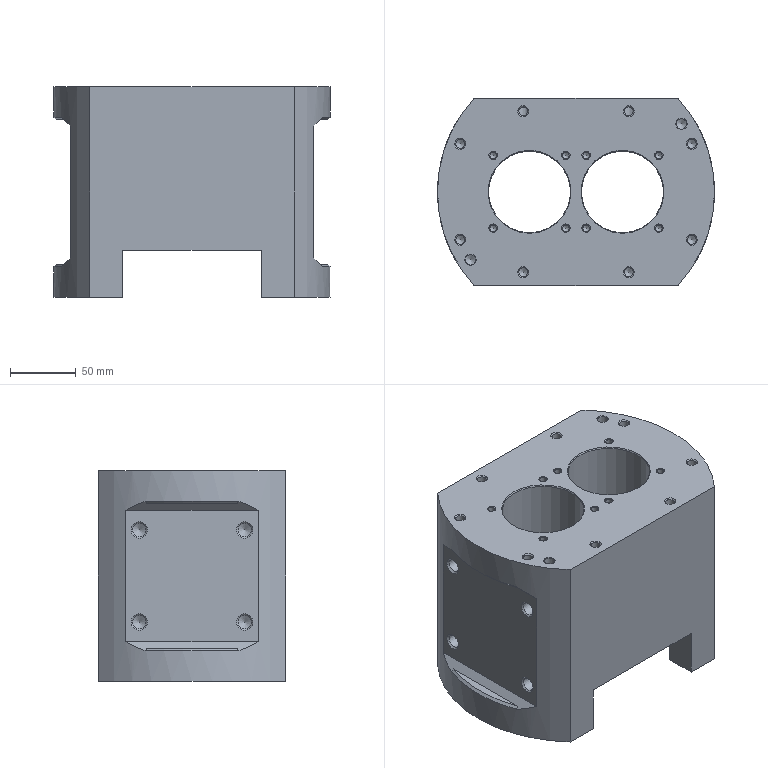NC program | NX | posted with a generic post | part box 210 x 142 x 160 mm
Whole program, first 1083 of 1408 lines:
N10 G17 G21 G94 G90
(FLOOR_WALL_COPY_COPY_COPY_COPY_1 , TOOL : D50)
N12 T02 M6
N14 G54
N16 G17 G0 G90 X-133. Y56.07 B0. C0. S2500 M3
N18 G43 Z30. H2
N20 Z4.
N22 G94 G1 Y70.997 Z0. F1000.
N24 X-108.901
N26 X108.901
N28 G2 X123.531 Y40.498 R130.
N30 G1 X-123.531
N32 G3 X-129.615 Y9.999 R130.
N34 G1 X129.615
N36 G2 X130. Y0.007 R130.
N38 G1 Y-0.007
N40 G2 X128.373 Y-20.501 R130.
N42 G1 X-128.373
N44 G3 X-119.578 Y-51. R130.
N46 G1 X119.578
N48 X122.578
N50 Z3.
N52 G0 Z30.
N54 M5
(DRILLING_COPY_2 , TOOL : ZXZ)
N56 T01 M6
N58 G54
N60 G17 G0 G90 X-87.769 Y36.355 B0. C0. S5000 M3
N62 G43 Z30. H1
N64 G94 G81 G98 Z-1. F250. R3.
N66 X-62.827 Y27.577
N68 X-40. Y61.
N70 X-7.673 Y27.577
N72 X7.673
N74 X40. Y61.
N76 X80. Y51.5
N78 X87.769 Y36.355
N80 X62.827 Y27.577
N82 X35.25 Y0.
N84 X62.827 Y-27.577
N86 X87.769 Y-36.355
N88 X40. Y-61.
N90 X7.673 Y-27.577
N92 X-7.673
N94 X-35.25 Y0.
N96 X-62.827 Y-27.577
N98 X-87.769 Y-36.355
N100 X-80. Y-51.5
N102 X-40. Y-61.
N104 G80
N106 G0 X-40. Y-61. Z30.
N108 M5
(DRILLING_COPY_2_COPY , TOOL : 6.8ZT)
N110 T16 M6
N112 G54
N114 G17 G0 G90 X-40. Y61. B0. C0. S2000 M3
N116 G43 Z30. H16
N118 G94 G83 G98 Z-24.742 F200. Q2. R3.
N120 X-87.769 Y36.355 Z-27.043
N122 Y-36.355
N124 X-40. Y-61.
N126 X40.
N128 X87.769 Y-36.355
N130 Y36.355
N132 X40. Y61. Z-24.742
N134 G80
N136 G0 X40. Y61. Z30.
N138 M5
(DRILLING_COPY_2_COPY_COPY_1 , TOOL : 5.2ZT)
N140 T15 M6
N142 G54
N144 G17 G0 G90 X62.827 Y27.577 B0. C0. S2000 M3
N146 G43 Z30. H15
N148 G94 G83 G98 Z-21.502 F200. Q2. R3.
N150 Y-27.577
N152 X7.673
N154 X-7.673
N156 X-62.827
N158 Y27.577
N160 X-7.673
N162 X7.673
N164 G80
N166 G0 X7.673 Y27.577 Z30.
N168 M5
(DRILLING_COPY_2_COPY_COPY_1_COPY_1 , TOOL : 7.8ZT)
N170 T17 M6
N172 G54
N174 G17 G0 G90 X80. Y51.5 B0. C0. S2000 M3
N176 G43 Z30. H17
N178 G94 G83 G98 Z-22.403 F200. Q2. R3.
N180 X-80. Y-51.5
N182 G80
N184 G0 X-80. Y-51.5 Z30.
N186 M5
(DRILLING_COPY_2_COPY_COPY_1_COPY_1_COPY , TOOL : 8.0JD)
N188 T18 M6
N190 G54
N192 G17 G0 G90 X80. Y51.5 B0. C0. S1000 M3
N194 G43 Z30. H18
N196 G94 G85 G98 Z-20. F40. R3.
N198 X-80. Y-51.5
N200 G80
N202 G0 X-80. Y-51.5 Z30.
N204 M5
(DRILLING_COPY_COPY_1_COPY , TOOL : 11.8ZT)
N206 T19 M6
N208 G54
N210 G17 G0 G90 X-35.25 Y0. B0. C0. S1025 M3
N212 G43 Z30. H19
N214 G94 G83 G98 Z-129.045 F150. Q2. R3.
N216 X35.25
N218 G80
N220 G0 X35.25 Y0. Z30.
N222 M5
(HOLE_MILLING , TOOL : D35R.5)
N224 T09 M6
N226 G54
N228 G17 G0 G90 X-35.25 Y0. B0. C0. S1500 M3
N230 G43 Z30. H9
N232 Z1.
N234 G94 G3 X-28.575 Y-6.675 R6.675 F1200.
N236 X-21.9 Y0. R6.675
N238 X-21.9 Y0. Z0.75 I-13.35 J0.
N240 X-21.9 Y0. Z0.5 I-13.35 J0.
N242 X-21.9 Y0. Z0.25 I-13.35 J0.
N244 X-21.9 Y0. Z0. I-13.35 J0.
N246 X-21.9 Y0. Z-0.25 I-13.35 J0.
N248 X-21.9 Y0. Z-0.5 I-13.35 J0.
N250 X-21.9 Y0. Z-0.75 I-13.35 J0.
N252 X-21.9 Y0. Z-1. I-13.35 J0.
N254 X-21.9 Y0. Z-1.25 I-13.35 J0.
N256 X-21.9 Y0. Z-1.5 I-13.35 J0.
N258 X-21.9 Y0. Z-1.75 I-13.35 J0.
N260 X-21.9 Y0. Z-2. I-13.35 J0.
N262 X-21.9 Y0. Z-2.25 I-13.35 J0.
N264 X-21.9 Y0. Z-2.5 I-13.35 J0.
N266 X-21.9 Y0. Z-2.75 I-13.35 J0.
N268 X-21.9 Y0. Z-3. I-13.35 J0.
N270 X-21.9 Y0. Z-3.25 I-13.35 J0.
N272 X-21.9 Y0. Z-3.5 I-13.35 J0.
N274 X-21.9 Y0. Z-3.75 I-13.35 J0.
N276 X-21.9 Y0. Z-4. I-13.35 J0.
N278 X-21.9 Y0. Z-4.25 I-13.35 J0.
N280 X-21.9 Y0. Z-4.5 I-13.35 J0.
N282 X-21.9 Y0. Z-4.75 I-13.35 J0.
N284 X-21.9 Y0. Z-5. I-13.35 J0.
N286 X-21.9 Y0. Z-5.25 I-13.35 J0.
N288 X-21.9 Y0. Z-5.5 I-13.35 J0.
N290 X-21.9 Y0. Z-5.75 I-13.35 J0.
N292 X-21.9 Y0. Z-6. I-13.35 J0.
N294 X-21.9 Y0. Z-6.25 I-13.35 J0.
N296 X-21.9 Y0. Z-6.5 I-13.35 J0.
N298 X-21.9 Y0. Z-6.75 I-13.35 J0.
N300 X-21.9 Y0. Z-7. I-13.35 J0.
N302 X-21.9 Y0. Z-7.25 I-13.35 J0.
N304 X-21.9 Y0. Z-7.5 I-13.35 J0.
N306 X-21.9 Y0. Z-7.75 I-13.35 J0.
N308 X-21.9 Y0. Z-8. I-13.35 J0.
N310 X-21.9 Y0. Z-8.25 I-13.35 J0.
N312 X-21.9 Y0. Z-8.5 I-13.35 J0.
N314 X-21.9 Y0. Z-8.75 I-13.35 J0.
N316 X-21.9 Y0. Z-9. I-13.35 J0.
N318 X-21.9 Y0. Z-9.25 I-13.35 J0.
N320 X-21.9 Y0. Z-9.5 I-13.35 J0.
N322 X-21.9 Y0. Z-9.75 I-13.35 J0.
N324 X-21.9 Y0. Z-10. I-13.35 J0.
N326 X-21.9 Y0. Z-10.25 I-13.35 J0.
N328 X-21.9 Y0. Z-10.5 I-13.35 J0.
N330 X-21.9 Y0. Z-10.75 I-13.35 J0.
N332 X-21.9 Y0. Z-11. I-13.35 J0.
N334 X-21.9 Y0. Z-11.25 I-13.35 J0.
N336 X-21.9 Y0. Z-11.5 I-13.35 J0.
N338 X-21.9 Y0. Z-11.75 I-13.35 J0.
N340 X-21.9 Y0. Z-12. I-13.35 J0.
N342 X-21.9 Y0. Z-12.25 I-13.35 J0.
N344 X-21.9 Y0. Z-12.5 I-13.35 J0.
N346 X-21.9 Y0. Z-12.75 I-13.35 J0.
N348 X-21.9 Y0. Z-13. I-13.35 J0.
N350 X-21.9 Y0. Z-13.25 I-13.35 J0.
N352 X-21.9 Y0. Z-13.5 I-13.35 J0.
N354 X-21.9 Y0. Z-13.75 I-13.35 J0.
N356 X-21.9 Y0. Z-14. I-13.35 J0.
N358 X-21.9 Y0. Z-14.25 I-13.35 J0.
N360 X-21.9 Y0. Z-14.5 I-13.35 J0.
N362 X-21.9 Y0. Z-14.75 I-13.35 J0.
N364 X-21.9 Y0. Z-15. I-13.35 J0.
N366 X-21.9 Y0. Z-15.25 I-13.35 J0.
N368 X-21.9 Y0. Z-15.5 I-13.35 J0.
N370 X-21.9 Y0. Z-15.75 I-13.35 J0.
N372 X-21.9 Y0. Z-16. I-13.35 J0.
N374 X-21.9 Y0. Z-16.25 I-13.35 J0.
N376 X-21.9 Y0. Z-16.5 I-13.35 J0.
N378 X-21.9 Y0. Z-16.75 I-13.35 J0.
N380 X-21.9 Y0. Z-17. I-13.35 J0.
N382 X-21.9 Y0. Z-17.25 I-13.35 J0.
N384 X-21.9 Y0. Z-17.5 I-13.35 J0.
N386 X-21.9 Y0. Z-17.75 I-13.35 J0.
N388 X-21.9 Y0. Z-18. I-13.35 J0.
N390 X-21.9 Y0. Z-18.25 I-13.35 J0.
N392 X-21.9 Y0. Z-18.5 I-13.35 J0.
N394 X-21.9 Y0. Z-18.75 I-13.35 J0.
N396 X-21.9 Y0. Z-19. I-13.35 J0.
N398 X-21.9 Y0. Z-19.25 I-13.35 J0.
N400 X-21.9 Y0. Z-19.5 I-13.35 J0.
N402 X-21.9 Y0. Z-19.75 I-13.35 J0.
N404 X-21.9 Y0. Z-20. I-13.35 J0.
N406 X-21.9 Y0. Z-20.25 I-13.35 J0.
N408 X-21.9 Y0. Z-20.5 I-13.35 J0.
N410 X-21.9 Y0. Z-20.75 I-13.35 J0.
N412 X-21.9 Y0. Z-21. I-13.35 J0.
N414 X-21.9 Y0. Z-21.25 I-13.35 J0.
N416 X-21.9 Y0. Z-21.5 I-13.35 J0.
N418 X-21.9 Y0. Z-21.75 I-13.35 J0.
N420 X-21.9 Y0. Z-22. I-13.35 J0.
N422 X-21.9 Y0. Z-22.25 I-13.35 J0.
N424 X-21.9 Y0. Z-22.5 I-13.35 J0.
N426 X-21.9 Y0. Z-22.75 I-13.35 J0.
N428 X-21.9 Y0. Z-23. I-13.35 J0.
N430 X-21.9 Y0. Z-23.25 I-13.35 J0.
N432 X-21.9 Y0. Z-23.5 I-13.35 J0.
N434 X-21.9 Y0. Z-23.75 I-13.35 J0.
N436 X-21.9 Y0. Z-24. I-13.35 J0.
N438 X-21.9 Y0. Z-24.25 I-13.35 J0.
N440 X-21.9 Y0. Z-24.5 I-13.35 J0.
N442 X-21.9 Y0. Z-24.75 I-13.35 J0.
N444 X-21.9 Y0. Z-25. I-13.35 J0.
N446 X-21.9 Y0. Z-25.25 I-13.35 J0.
N448 X-21.9 Y0. Z-25.5 I-13.35 J0.
N450 X-21.9 Y0. Z-25.75 I-13.35 J0.
N452 X-21.9 Y0. Z-26. I-13.35 J0.
N454 X-21.9 Y0. Z-26.25 I-13.35 J0.
N456 X-21.9 Y0. Z-26.5 I-13.35 J0.
N458 X-21.9 Y0. Z-26.75 I-13.35 J0.
N460 X-21.9 Y0. Z-27. I-13.35 J0.
N462 X-21.9 Y0. Z-27.25 I-13.35 J0.
N464 X-21.9 Y0. Z-27.5 I-13.35 J0.
N466 X-21.9 Y0. Z-27.75 I-13.35 J0.
N468 X-21.9 Y0. Z-28. I-13.35 J0.
N470 X-21.9 Y0. Z-28.25 I-13.35 J0.
N472 X-21.9 Y0. Z-28.5 I-13.35 J0.
N474 X-21.9 Y0. Z-28.75 I-13.35 J0.
N476 X-21.9 Y0. Z-29. I-13.35 J0.
N478 X-21.9 Y0. Z-29.25 I-13.35 J0.
N480 X-21.9 Y0. Z-29.5 I-13.35 J0.
N482 X-21.9 Y0. Z-29.75 I-13.35 J0.
N484 X-21.9 Y0. Z-30. I-13.35 J0.
N486 X-21.9 Y0. Z-30.25 I-13.35 J0.
N488 X-21.9 Y0. Z-30.5 I-13.35 J0.
N490 X-21.9 Y0. Z-30.75 I-13.35 J0.
N492 X-21.9 Y0. Z-31. I-13.35 J0.
N494 X-21.9 Y0. Z-31.25 I-13.35 J0.
N496 X-21.9 Y0. Z-31.5 I-13.35 J0.
N498 X-21.9 Y0. Z-31.75 I-13.35 J0.
N500 X-21.9 Y0. Z-32. I-13.35 J0.
N502 X-21.9 Y0. Z-32.25 I-13.35 J0.
N504 X-21.9 Y0. Z-32.5 I-13.35 J0.
N506 X-21.9 Y0. Z-32.75 I-13.35 J0.
N508 X-21.9 Y0. Z-33. I-13.35 J0.
N510 X-21.9 Y0. Z-33.25 I-13.35 J0.
N512 X-21.9 Y0. Z-33.5 I-13.35 J0.
N514 X-21.9 Y0. Z-33.75 I-13.35 J0.
N516 X-21.9 Y0. Z-34. I-13.35 J0.
N518 X-21.9 Y0. Z-34.25 I-13.35 J0.
N520 X-21.9 Y0. Z-34.5 I-13.35 J0.
N522 X-21.9 Y0. Z-34.75 I-13.35 J0.
N524 X-21.9 Y0. Z-35. I-13.35 J0.
N526 X-21.9 Y0. Z-35.25 I-13.35 J0.
N528 X-21.9 Y0. Z-35.5 I-13.35 J0.
N530 X-21.9 Y0. Z-35.75 I-13.35 J0.
N532 X-21.9 Y0. Z-36. I-13.35 J0.
N534 X-21.9 Y0. Z-36.25 I-13.35 J0.
N536 X-21.9 Y0. Z-36.5 I-13.35 J0.
N538 X-21.9 Y0. Z-36.75 I-13.35 J0.
N540 X-21.9 Y0. Z-37. I-13.35 J0.
N542 X-21.9 Y0. Z-37.25 I-13.35 J0.
N544 X-21.9 Y0. Z-37.5 I-13.35 J0.
N546 X-21.9 Y0. Z-37.75 I-13.35 J0.
N548 X-21.9 Y0. Z-38. I-13.35 J0.
N550 X-21.9 Y0. Z-38.25 I-13.35 J0.
N552 X-21.9 Y0. Z-38.5 I-13.35 J0.
N554 X-21.9 Y0. Z-38.75 I-13.35 J0.
N556 X-21.9 Y0. Z-39. I-13.35 J0.
N558 X-21.9 Y0. Z-39.25 I-13.35 J0.
N560 X-21.9 Y0. Z-39.5 I-13.35 J0.
N562 X-21.9 Y0. Z-39.75 I-13.35 J0.
N564 X-21.9 Y0. Z-40. I-13.35 J0.
N566 X-21.9 Y0. Z-40.25 I-13.35 J0.
N568 X-21.9 Y0. Z-40.5 I-13.35 J0.
N570 X-21.9 Y0. Z-40.75 I-13.35 J0.
N572 X-21.9 Y0. Z-41. I-13.35 J0.
N574 X-21.9 Y0. Z-41.25 I-13.35 J0.
N576 X-21.9 Y0. Z-41.5 I-13.35 J0.
N578 X-21.9 Y0. Z-41.75 I-13.35 J0.
N580 X-21.9 Y0. Z-42. I-13.35 J0.
N582 X-21.9 Y0. Z-42.25 I-13.35 J0.
N584 X-21.9 Y0. Z-42.5 I-13.35 J0.
N586 X-21.9 Y0. Z-42.75 I-13.35 J0.
N588 X-21.9 Y0. Z-43. I-13.35 J0.
N590 X-21.9 Y0. Z-43.25 I-13.35 J0.
N592 X-21.9 Y0. Z-43.5 I-13.35 J0.
N594 X-21.9 Y0. Z-43.75 I-13.35 J0.
N596 X-21.9 Y0. Z-44. I-13.35 J0.
N598 X-21.9 Y0. Z-44.25 I-13.35 J0.
N600 X-21.9 Y0. Z-44.5 I-13.35 J0.
N602 X-21.9 Y0. Z-44.75 I-13.35 J0.
N604 X-21.9 Y0. Z-45. I-13.35 J0.
N606 X-21.9 Y0. Z-45.25 I-13.35 J0.
N608 X-21.9 Y0. Z-45.5 I-13.35 J0.
N610 X-21.9 Y0. Z-45.75 I-13.35 J0.
N612 X-21.9 Y0. Z-46. I-13.35 J0.
N614 X-21.9 Y0. Z-46.25 I-13.35 J0.
N616 X-21.9 Y0. Z-46.5 I-13.35 J0.
N618 X-21.9 Y0. Z-46.75 I-13.35 J0.
N620 X-21.9 Y0. Z-47. I-13.35 J0.
N622 X-21.9 Y0. Z-47.25 I-13.35 J0.
N624 X-21.9 Y0. Z-47.5 I-13.35 J0.
N626 X-21.9 Y0. Z-47.75 I-13.35 J0.
N628 X-21.9 Y0. Z-48. I-13.35 J0.
N630 X-21.9 Y0. Z-48.25 I-13.35 J0.
N632 X-21.9 Y0. Z-48.5 I-13.35 J0.
N634 X-21.9 Y0. Z-48.75 I-13.35 J0.
N636 X-21.9 Y0. Z-49. I-13.35 J0.
N638 X-21.9 Y0. Z-49.25 I-13.35 J0.
N640 X-21.9 Y0. Z-49.5 I-13.35 J0.
N642 X-21.9 Y0. Z-49.75 I-13.35 J0.
N644 X-21.9 Y0. Z-50. I-13.35 J0.
N646 X-21.9 Y0. Z-50.25 I-13.35 J0.
N648 X-21.9 Y0. Z-50.5 I-13.35 J0.
N650 X-21.9 Y0. Z-50.75 I-13.35 J0.
N652 X-21.9 Y0. Z-51. I-13.35 J0.
N654 X-21.9 Y0. Z-51.25 I-13.35 J0.
N656 X-21.9 Y0. Z-51.5 I-13.35 J0.
N658 X-21.9 Y0. Z-51.75 I-13.35 J0.
N660 X-21.9 Y0. Z-52. I-13.35 J0.
N662 X-21.9 Y0. Z-52.25 I-13.35 J0.
N664 X-21.9 Y0. Z-52.5 I-13.35 J0.
N666 X-21.9 Y0. Z-52.75 I-13.35 J0.
N668 X-21.9 Y0. Z-53. I-13.35 J0.
N670 X-21.9 Y0. Z-53.25 I-13.35 J0.
N672 X-21.9 Y0. Z-53.5 I-13.35 J0.
N674 X-21.9 Y0. Z-53.75 I-13.35 J0.
N676 X-21.9 Y0. Z-54. I-13.35 J0.
N678 X-21.9 Y0. Z-54.25 I-13.35 J0.
N680 X-21.9 Y0. Z-54.5 I-13.35 J0.
N682 X-21.9 Y0. Z-54.75 I-13.35 J0.
N684 X-21.9 Y0. Z-55. I-13.35 J0.
N686 X-21.9 Y0. Z-55.25 I-13.35 J0.
N688 X-21.9 Y0. Z-55.5 I-13.35 J0.
N690 X-21.9 Y0. Z-55.75 I-13.35 J0.
N692 X-21.9 Y0. Z-56. I-13.35 J0.
N694 X-21.9 Y0. Z-56.25 I-13.35 J0.
N696 X-21.9 Y0. Z-56.5 I-13.35 J0.
N698 X-21.9 Y0. Z-56.75 I-13.35 J0.
N700 X-21.9 Y0. Z-57. I-13.35 J0.
N702 X-21.9 Y0. Z-57.25 I-13.35 J0.
N704 X-21.9 Y0. Z-57.5 I-13.35 J0.
N706 X-21.9 Y0. Z-57.75 I-13.35 J0.
N708 X-21.9 Y0. Z-58. I-13.35 J0.
N710 X-21.9 Y0. Z-58.25 I-13.35 J0.
N712 X-21.9 Y0. Z-58.5 I-13.35 J0.
N714 X-21.9 Y0. Z-58.75 I-13.35 J0.
N716 X-21.9 Y0. Z-59. I-13.35 J0.
N718 X-21.9 Y0. Z-59.25 I-13.35 J0.
N720 X-21.9 Y0. Z-59.5 I-13.35 J0.
N722 X-21.9 Y0. Z-59.75 I-13.35 J0.
N724 X-21.9 Y0. Z-60. I-13.35 J0.
N726 X-21.9 Y0. Z-60.25 I-13.35 J0.
N728 X-21.9 Y0. Z-60.5 I-13.35 J0.
N730 X-21.9 Y0. Z-60.75 I-13.35 J0.
N732 X-21.9 Y0. Z-61. I-13.35 J0.
N734 X-21.9 Y0. Z-61.25 I-13.35 J0.
N736 X-21.9 Y0. Z-61.5 I-13.35 J0.
N738 X-21.9 Y0. Z-61.75 I-13.35 J0.
N740 X-21.9 Y0. Z-62. I-13.35 J0.
N742 X-21.9 Y0. Z-62.25 I-13.35 J0.
N744 X-21.9 Y0. Z-62.5 I-13.35 J0.
N746 X-21.9 Y0. Z-62.75 I-13.35 J0.
N748 X-21.9 Y0. Z-63. I-13.35 J0.
N750 X-21.9 Y0. Z-63.25 I-13.35 J0.
N752 X-21.9 Y0. Z-63.5 I-13.35 J0.
N754 X-21.9 Y0. Z-63.75 I-13.35 J0.
N756 X-21.9 Y0. Z-64. I-13.35 J0.
N758 X-21.9 Y0. Z-64.25 I-13.35 J0.
N760 X-21.9 Y0. Z-64.5 I-13.35 J0.
N762 X-21.9 Y0. Z-64.75 I-13.35 J0.
N764 X-21.9 Y0. Z-65. I-13.35 J0.
N766 X-21.9 Y0. Z-65.25 I-13.35 J0.
N768 X-21.9 Y0. Z-65.5 I-13.35 J0.
N770 X-21.9 Y0. Z-65.75 I-13.35 J0.
N772 X-21.9 Y0. Z-66. I-13.35 J0.
N774 X-21.9 Y0. Z-66.25 I-13.35 J0.
N776 X-21.9 Y0. Z-66.5 I-13.35 J0.
N778 X-21.9 Y0. Z-66.75 I-13.35 J0.
N780 X-21.9 Y0. Z-67. I-13.35 J0.
N782 X-21.9 Y0. Z-67.25 I-13.35 J0.
N784 X-21.9 Y0. Z-67.5 I-13.35 J0.
N786 X-21.9 Y0. Z-67.75 I-13.35 J0.
N788 X-21.9 Y0. Z-68. I-13.35 J0.
N790 X-21.9 Y0. Z-68.25 I-13.35 J0.
N792 X-21.9 Y0. Z-68.5 I-13.35 J0.
N794 X-21.9 Y0. Z-68.75 I-13.35 J0.
N796 X-21.9 Y0. Z-69. I-13.35 J0.
N798 X-21.9 Y0. Z-69.25 I-13.35 J0.
N800 X-21.9 Y0. Z-69.5 I-13.35 J0.
N802 X-21.9 Y0. Z-69.75 I-13.35 J0.
N804 X-21.9 Y0. Z-70. I-13.35 J0.
N806 X-21.9 Y0. Z-70.25 I-13.35 J0.
N808 X-21.9 Y0. Z-70.5 I-13.35 J0.
N810 X-21.9 Y0. Z-70.75 I-13.35 J0.
N812 X-21.9 Y0. Z-71. I-13.35 J0.
N814 X-21.9 Y0. Z-71.25 I-13.35 J0.
N816 X-21.9 Y0. Z-71.5 I-13.35 J0.
N818 X-21.9 Y0. Z-71.75 I-13.35 J0.
N820 X-21.9 Y0. Z-72. I-13.35 J0.
N822 X-21.9 Y0. Z-72.25 I-13.35 J0.
N824 X-21.9 Y0. Z-72.5 I-13.35 J0.
N826 X-21.9 Y0. Z-72.75 I-13.35 J0.
N828 X-21.9 Y0. Z-73. I-13.35 J0.
N830 X-21.9 Y0. Z-73.25 I-13.35 J0.
N832 X-21.9 Y0. Z-73.5 I-13.35 J0.
N834 X-21.9 Y0. Z-73.75 I-13.35 J0.
N836 X-21.9 Y0. Z-74. I-13.35 J0.
N838 X-21.9 Y0. Z-74.25 I-13.35 J0.
N840 X-21.9 Y0. Z-74.5 I-13.35 J0.
N842 X-21.9 Y0. Z-74.75 I-13.35 J0.
N844 X-21.9 Y0. Z-75. I-13.35 J0.
N846 X-21.9 Y0. Z-75.25 I-13.35 J0.
N848 X-21.9 Y0. Z-75.5 I-13.35 J0.
N850 X-21.9 Y0. Z-75.75 I-13.35 J0.
N852 X-21.9 Y0. Z-76. I-13.35 J0.
N854 X-21.9 Y0. Z-76.25 I-13.35 J0.
N856 X-21.9 Y0. Z-76.5 I-13.35 J0.
N858 X-21.9 Y0. Z-76.75 I-13.35 J0.
N860 X-21.9 Y0. Z-77. I-13.35 J0.
N862 X-21.9 Y0. Z-77.25 I-13.35 J0.
N864 X-21.9 Y0. Z-77.5 I-13.35 J0.
N866 X-21.9 Y0. Z-77.75 I-13.35 J0.
N868 X-21.9 Y0. Z-78. I-13.35 J0.
N870 X-21.9 Y0. Z-78.25 I-13.35 J0.
N872 X-21.9 Y0. Z-78.5 I-13.35 J0.
N874 X-21.9 Y0. Z-78.75 I-13.35 J0.
N876 X-21.9 Y0. Z-79. I-13.35 J0.
N878 X-21.9 Y0. Z-79.25 I-13.35 J0.
N880 X-21.9 Y0. Z-79.5 I-13.35 J0.
N882 X-21.9 Y0. Z-79.75 I-13.35 J0.
N884 X-21.9 Y0. Z-80. I-13.35 J0.
N886 X-21.9 Y0. Z-80.25 I-13.35 J0.
N888 X-21.9 Y0. Z-80.5 I-13.35 J0.
N890 X-21.9 Y0. Z-80.75 I-13.35 J0.
N892 X-21.9 Y0. Z-81. I-13.35 J0.
N894 X-21.9 Y0. Z-81.25 I-13.35 J0.
N896 X-21.9 Y0. Z-81.5 I-13.35 J0.
N898 X-21.9 Y0. Z-81.75 I-13.35 J0.
N900 X-21.9 Y0. Z-82. I-13.35 J0.
N902 X-21.9 Y0. Z-82.25 I-13.35 J0.
N904 X-21.9 Y0. Z-82.5 I-13.35 J0.
N906 X-21.9 Y0. Z-82.75 I-13.35 J0.
N908 X-21.9 Y0. Z-83. I-13.35 J0.
N910 X-21.9 Y0. Z-83.25 I-13.35 J0.
N912 X-21.9 Y0. Z-83.5 I-13.35 J0.
N914 X-21.9 Y0. Z-83.75 I-13.35 J0.
N916 X-21.9 Y0. Z-84. I-13.35 J0.
N918 X-21.9 Y0. Z-84.25 I-13.35 J0.
N920 X-21.9 Y0. Z-84.5 I-13.35 J0.
N922 X-21.9 Y0. Z-84.75 I-13.35 J0.
N924 X-21.9 Y0. Z-85. I-13.35 J0.
N926 X-21.9 Y0. Z-85.25 I-13.35 J0.
N928 X-21.9 Y0. Z-85.5 I-13.35 J0.
N930 X-21.9 Y0. Z-85.75 I-13.35 J0.
N932 X-21.9 Y0. Z-86. I-13.35 J0.
N934 X-21.9 Y0. Z-86.25 I-13.35 J0.
N936 X-21.9 Y0. Z-86.5 I-13.35 J0.
N938 X-21.9 Y0. Z-86.75 I-13.35 J0.
N940 X-21.9 Y0. Z-87. I-13.35 J0.
N942 X-21.9 Y0. Z-87.25 I-13.35 J0.
N944 X-21.9 Y0. Z-87.5 I-13.35 J0.
N946 X-21.9 Y0. Z-87.75 I-13.35 J0.
N948 X-21.9 Y0. Z-88. I-13.35 J0.
N950 X-21.9 Y0. Z-88.25 I-13.35 J0.
N952 X-21.9 Y0. Z-88.5 I-13.35 J0.
N954 X-21.9 Y0. Z-88.75 I-13.35 J0.
N956 X-21.9 Y0. Z-89. I-13.35 J0.
N958 X-21.9 Y0. Z-89.25 I-13.35 J0.
N960 X-21.9 Y0. Z-89.5 I-13.35 J0.
N962 X-21.9 Y0. Z-89.75 I-13.35 J0.
N964 X-21.9 Y0. Z-90. I-13.35 J0.
N966 X-21.9 Y0. Z-90.25 I-13.35 J0.
N968 X-21.9 Y0. Z-90.5 I-13.35 J0.
N970 X-21.9 Y0. Z-90.75 I-13.35 J0.
N972 X-21.9 Y0. Z-91. I-13.35 J0.
N974 X-21.9 Y0. Z-91.25 I-13.35 J0.
N976 X-21.9 Y0. Z-91.5 I-13.35 J0.
N978 X-21.9 Y0. Z-91.75 I-13.35 J0.
N980 X-21.9 Y0. Z-92. I-13.35 J0.
N982 X-21.9 Y0. Z-92.25 I-13.35 J0.
N984 X-21.9 Y0. Z-92.5 I-13.35 J0.
N986 X-21.9 Y0. Z-92.75 I-13.35 J0.
N988 X-21.9 Y0. Z-93. I-13.35 J0.
N990 X-21.9 Y0. Z-93.25 I-13.35 J0.
N992 X-21.9 Y0. Z-93.5 I-13.35 J0.
N994 X-21.9 Y0. Z-93.75 I-13.35 J0.
N996 X-21.9 Y0. Z-94. I-13.35 J0.
N998 X-21.9 Y0. Z-94.25 I-13.35 J0.
N1000 X-21.9 Y0. Z-94.5 I-13.35 J0.
N1002 X-21.9 Y0. Z-94.75 I-13.35 J0.
N1004 X-21.9 Y0. Z-95. I-13.35 J0.
N1006 X-21.9 Y0. Z-95.25 I-13.35 J0.
N1008 X-21.9 Y0. Z-95.5 I-13.35 J0.
N1010 X-21.9 Y0. Z-95.75 I-13.35 J0.
N1012 X-21.9 Y0. Z-96. I-13.35 J0.
N1014 X-21.9 Y0. Z-96.25 I-13.35 J0.
N1016 X-21.9 Y0. Z-96.5 I-13.35 J0.
N1018 X-21.9 Y0. Z-96.75 I-13.35 J0.
N1020 X-21.9 Y0. Z-97. I-13.35 J0.
N1022 X-21.9 Y0. Z-97.25 I-13.35 J0.
N1024 X-21.9 Y0. Z-97.5 I-13.35 J0.
N1026 X-21.9 Y0. Z-97.75 I-13.35 J0.
N1028 X-21.9 Y0. Z-98. I-13.35 J0.
N1030 X-21.9 Y0. Z-98.25 I-13.35 J0.
N1032 X-21.9 Y0. Z-98.5 I-13.35 J0.
N1034 X-21.9 Y0. Z-98.75 I-13.35 J0.
N1036 X-21.9 Y0. Z-99. I-13.35 J0.
N1038 X-21.9 Y0. Z-99.25 I-13.35 J0.
N1040 X-21.9 Y0. Z-99.5 I-13.35 J0.
N1042 X-21.9 Y0. Z-99.75 I-13.35 J0.
N1044 X-21.9 Y0. Z-100. I-13.35 J0.
N1046 X-21.9 Y0. Z-100.25 I-13.35 J0.
N1048 X-21.9 Y0. Z-100.5 I-13.35 J0.
N1050 X-21.9 Y0. Z-100.75 I-13.35 J0.
N1052 X-21.9 Y0. Z-101. I-13.35 J0.
N1054 X-21.9 Y0. Z-101.25 I-13.35 J0.
N1056 X-21.9 Y0. Z-101.5 I-13.35 J0.
N1058 X-21.9 Y0. Z-101.75 I-13.35 J0.
N1060 X-21.9 Y0. Z-102. I-13.35 J0.
N1062 X-21.9 Y0. Z-102.25 I-13.35 J0.
N1064 X-21.9 Y0. Z-102.5 I-13.35 J0.
N1066 X-21.9 Y0. Z-102.75 I-13.35 J0.
N1068 X-21.9 Y0. Z-103. I-13.35 J0.
N1070 X-21.9 Y0. Z-103.25 I-13.35 J0.
N1072 X-21.9 Y0. Z-103.5 I-13.35 J0.
N1074 X-21.9 Y0. Z-103.75 I-13.35 J0.
N1076 X-21.9 Y0. Z-104. I-13.35 J0.
N1078 X-21.9 Y0. Z-104.25 I-13.35 J0.
N1080 X-21.9 Y0. Z-104.5 I-13.35 J0.
N1082 X-21.9 Y0. Z-104.75 I-13.35 J0.
N1084 X-21.9 Y0. Z-105. I-13.35 J0.
N1086 X-21.9 Y0. Z-105.25 I-13.35 J0.
N1088 X-21.9 Y0. Z-105.5 I-13.35 J0.
N1090 X-21.9 Y0. Z-105.75 I-13.35 J0.
N1092 X-21.9 Y0. Z-106. I-13.35 J0.
N1094 X-21.9 Y0. Z-106.25 I-13.35 J0.
N1096 X-21.9 Y0. Z-106.5 I-13.35 J0.
N1098 X-21.9 Y0. Z-106.75 I-13.35 J0.
N1100 X-21.9 Y0. Z-107. I-13.35 J0.
N1102 X-21.9 Y0. Z-107.25 I-13.35 J0.
N1104 X-21.9 Y0. Z-107.5 I-13.35 J0.
N1106 X-21.9 Y0. Z-107.75 I-13.35 J0.
N1108 X-21.9 Y0. Z-108. I-13.35 J0.
N1110 X-21.9 Y0. Z-108.25 I-13.35 J0.
N1112 X-21.9 Y0. Z-108.5 I-13.35 J0.
N1114 X-21.9 Y0. Z-108.75 I-13.35 J0.
N1116 X-21.9 Y0. Z-109. I-13.35 J0.
N1118 X-21.9 Y0. Z-109.25 I-13.35 J0.
N1120 X-21.9 Y0. Z-109.5 I-13.35 J0.
N1122 X-21.9 Y0. Z-109.75 I-13.35 J0.
N1124 X-21.9 Y0. Z-110. I-13.35 J0.
N1126 X-21.9 Y0. Z-110.25 I-13.35 J0.
N1128 X-21.9 Y0. Z-110.5 I-13.35 J0.
N1130 X-21.9 Y0. Z-110.75 I-13.35 J0.
N1132 X-21.9 Y0. Z-111. I-13.35 J0.
N1134 X-21.9 Y0. Z-111.25 I-13.35 J0.
N1136 X-21.9 Y0. Z-111.5 I-13.35 J0.
N1138 X-21.9 Y0. Z-111.75 I-13.35 J0.
N1140 X-21.9 Y0. Z-112. I-13.35 J0.
N1142 X-21.9 Y0. Z-112.25 I-13.35 J0.
N1144 X-21.9 Y0. Z-112.5 I-13.35 J0.
N1146 X-21.9 Y0. Z-112.75 I-13.35 J0.
N1148 X-21.9 Y0. Z-113. I-13.35 J0.
N1150 X-21.9 Y0. Z-113.25 I-13.35 J0.
N1152 X-21.9 Y0. Z-113.5 I-13.35 J0.
N1154 X-21.9 Y0. Z-113.75 I-13.35 J0.
N1156 X-21.9 Y0. Z-114. I-13.35 J0.
N1158 X-21.9 Y0. Z-114.25 I-13.35 J0.
N1160 X-21.9 Y0. Z-114.5 I-13.35 J0.
N1162 X-21.9 Y0. Z-114.75 I-13.35 J0.
N1164 X-21.9 Y0. Z-115. I-13.35 J0.
N1166 X-21.9 Y0. Z-115.25 I-13.35 J0.
N1168 X-21.9 Y0. Z-115.5 I-13.35 J0.
N1170 X-21.9 Y0. Z-115.75 I-13.35 J0.
N1172 X-21.9 Y0. Z-116. I-13.35 J0.
N1174 X-21.9 Y0. Z-116.25 I-13.35 J0.
N1176 X-21.9 Y0. Z-116.5 I-13.35 J0.
N1178 X-21.9 Y0. Z-116.75 I-13.35 J0.
N1180 X-21.9 Y0. Z-117. I-13.35 J0.
N1182 X-21.9 Y0. Z-117.25 I-13.35 J0.
N1184 X-21.9 Y0. Z-117.5 I-13.35 J0.
N1186 X-21.9 Y0. Z-117.75 I-13.35 J0.
N1188 X-21.9 Y0. Z-118. I-13.35 J0.
N1190 X-21.9 Y0. Z-118.25 I-13.35 J0.
N1192 X-21.9 Y0. Z-118.5 I-13.35 J0.
N1194 X-21.9 Y0. Z-118.75 I-13.35 J0.
N1196 X-21.9 Y0. Z-119. I-13.35 J0.
N1198 X-21.9 Y0. Z-119.25 I-13.35 J0.
N1200 X-21.9 Y0. Z-119.5 I-13.35 J0.
N1202 X-21.9 Y0. Z-119.75 I-13.35 J0.
N1204 X-21.9 Y0. Z-120. I-13.35 J0.
N1206 X-21.9 Y0. Z-120.25 I-13.35 J0.
N1208 X-21.9 Y0. Z-120.5 I-13.35 J0.
N1210 X-21.9 Y0. Z-120.75 I-13.35 J0.
N1212 X-21.9 Y0. Z-121. I-13.35 J0.
N1214 X-21.9 Y0. Z-121.25 I-13.35 J0.
N1216 X-21.9 Y0. Z-121.5 I-13.35 J0.
N1218 X-21.9 Y0. Z-121.75 I-13.35 J0.
N1220 X-21.9 Y0. Z-122. I-13.35 J0.
N1222 X-21.9 Y0. Z-122.25 I-13.35 J0.
N1224 X-21.9 Y0. Z-122.5 I-13.35 J0.
N1226 X-21.9 Y0. Z-122.75 I-13.35 J0.
N1228 X-21.9 Y0. Z-123. I-13.35 J0.
N1230 X-21.9 Y0. Z-123.25 I-13.35 J0.
N1232 X-21.9 Y0. Z-123.5 I-13.35 J0.
N1234 X-21.9 Y0. Z-123.75 I-13.35 J0.
N1236 X-21.9 Y0. Z-124. I-13.35 J0.
N1238 X-21.9 Y0. Z-124.25 I-13.35 J0.
N1240 X-21.9 Y0. Z-124.5 I-13.35 J0.
N1242 X-21.9 Y0. Z-124.75 I-13.35 J0.
N1244 X-21.9 Y0. Z-125. I-13.35 J0.
N1246 X-21.9 Y0. Z-125.25 I-13.35 J0.
N1248 X-21.9 Y0. Z-125.5 I-13.35 J0.
N1250 X-21.9 Y0. Z-125.75 I-13.35 J0.
N1252 X-21.9 Y0. Z-126. I-13.35 J0.
N1254 X-35.25 Y13.35 R13.35
N1256 X-21.9 Y0. R-13.35
N1258 X-28.575 Y6.675 R6.675
N1260 X-35.25 Y0. R6.675
N1262 G0 Z30.
N1264 X35.25
N1266 Z1.
N1268 G3 X41.925 Y-6.675 R6.675
N1270 X48.6 Y0. R6.675
N1272 X48.6 Y0. Z0.75 I-13.35 J0.
N1274 X48.6 Y0. Z0.5 I-13.35 J0.
N1276 X48.6 Y0. Z0.25 I-13.35 J0.
N1278 X48.6 Y0. Z0. I-13.35 J0.
N1280 X48.6 Y0. Z-0.25 I-13.35 J0.
N1282 X48.6 Y0. Z-0.5 I-13.35 J0.
N1284 X48.6 Y0. Z-0.75 I-13.35 J0.
N1286 X48.6 Y0. Z-1. I-13.35 J0.
N1288 X48.6 Y0. Z-1.25 I-13.35 J0.
N1290 X48.6 Y0. Z-1.5 I-13.35 J0.
N1292 X48.6 Y0. Z-1.75 I-13.35 J0.
N1294 X48.6 Y0. Z-2. I-13.35 J0.
N1296 X48.6 Y0. Z-2.25 I-13.35 J0.
N1298 X48.6 Y0. Z-2.5 I-13.35 J0.
N1300 X48.6 Y0. Z-2.75 I-13.35 J0.
N1302 X48.6 Y0. Z-3. I-13.35 J0.
N1304 X48.6 Y0. Z-3.25 I-13.35 J0.
N1306 X48.6 Y0. Z-3.5 I-13.35 J0.
N1308 X48.6 Y0. Z-3.75 I-13.35 J0.
N1310 X48.6 Y0. Z-4. I-13.35 J0.
N1312 X48.6 Y0. Z-4.25 I-13.35 J0.
N1314 X48.6 Y0. Z-4.5 I-13.35 J0.
N1316 X48.6 Y0. Z-4.75 I-13.35 J0.
N1318 X48.6 Y0. Z-5. I-13.35 J0.
N1320 X48.6 Y0. Z-5.25 I-13.35 J0.
N1322 X48.6 Y0. Z-5.5 I-13.35 J0.
N1324 X48.6 Y0. Z-5.75 I-13.35 J0.
N1326 X48.6 Y0. Z-6. I-13.35 J0.
N1328 X48.6 Y0. Z-6.25 I-13.35 J0.
N1330 X48.6 Y0. Z-6.5 I-13.35 J0.
N1332 X48.6 Y0. Z-6.75 I-13.35 J0.
N1334 X48.6 Y0. Z-7. I-13.35 J0.
N1336 X48.6 Y0. Z-7.25 I-13.35 J0.
N1338 X48.6 Y0. Z-7.5 I-13.35 J0.
N1340 X48.6 Y0. Z-7.75 I-13.35 J0.
N1342 X48.6 Y0. Z-8. I-13.35 J0.
N1344 X48.6 Y0. Z-8.25 I-13.35 J0.
N1346 X48.6 Y0. Z-8.5 I-13.35 J0.
N1348 X48.6 Y0. Z-8.75 I-13.35 J0.
N1350 X48.6 Y0. Z-9. I-13.35 J0.
N1352 X48.6 Y0. Z-9.25 I-13.35 J0.
N1354 X48.6 Y0. Z-9.5 I-13.35 J0.
N1356 X48.6 Y0. Z-9.75 I-13.35 J0.
N1358 X48.6 Y0. Z-10. I-13.35 J0.
N1360 X48.6 Y0. Z-10.25 I-13.35 J0.
N1362 X48.6 Y0. Z-10.5 I-13.35 J0.
N1364 X48.6 Y0. Z-10.75 I-13.35 J0.
N1366 X48.6 Y0. Z-11. I-13.35 J0.
N1368 X48.6 Y0. Z-11.25 I-13.35 J0.
N1370 X48.6 Y0. Z-11.5 I-13.35 J0.
N1372 X48.6 Y0. Z-11.75 I-13.35 J0.
N1374 X48.6 Y0. Z-12. I-13.35 J0.
N1376 X48.6 Y0. Z-12.25 I-13.35 J0.
N1378 X48.6 Y0. Z-12.5 I-13.35 J0.
N1380 X48.6 Y0. Z-12.75 I-13.35 J0.
N1382 X48.6 Y0. Z-13. I-13.35 J0.
N1384 X48.6 Y0. Z-13.25 I-13.35 J0.
N1386 X48.6 Y0. Z-13.5 I-13.35 J0.
N1388 X48.6 Y0. Z-13.75 I-13.35 J0.
N1390 X48.6 Y0. Z-14. I-13.35 J0.
N1392 X48.6 Y0. Z-14.25 I-13.35 J0.
N1394 X48.6 Y0. Z-14.5 I-13.35 J0.
N1396 X48.6 Y0. Z-14.75 I-13.35 J0.
N1398 X48.6 Y0. Z-15. I-13.35 J0.
N1400 X48.6 Y0. Z-15.25 I-13.35 J0.
N1402 X48.6 Y0. Z-15.5 I-13.35 J0.
N1404 X48.6 Y0. Z-15.75 I-13.35 J0.
N1406 X48.6 Y0. Z-16. I-13.35 J0.
N1408 X48.6 Y0. Z-16.25 I-13.35 J0.
N1410 X48.6 Y0. Z-16.5 I-13.35 J0.
N1412 X48.6 Y0. Z-16.75 I-13.35 J0.
N1414 X48.6 Y0. Z-17. I-13.35 J0.
N1416 X48.6 Y0. Z-17.25 I-13.35 J0.
N1418 X48.6 Y0. Z-17.5 I-13.35 J0.
N1420 X48.6 Y0. Z-17.75 I-13.35 J0.
N1422 X48.6 Y0. Z-18. I-13.35 J0.
N1424 X48.6 Y0. Z-18.25 I-13.35 J0.
N1426 X48.6 Y0. Z-18.5 I-13.35 J0.
N1428 X48.6 Y0. Z-18.75 I-13.35 J0.
N1430 X48.6 Y0. Z-19. I-13.35 J0.
N1432 X48.6 Y0. Z-19.25 I-13.35 J0.
N1434 X48.6 Y0. Z-19.5 I-13.35 J0.
N1436 X48.6 Y0. Z-19.75 I-13.35 J0.
N1438 X48.6 Y0. Z-20. I-13.35 J0.
N1440 X48.6 Y0. Z-20.25 I-13.35 J0.
N1442 X48.6 Y0. Z-20.5 I-13.35 J0.
N1444 X48.6 Y0. Z-20.75 I-13.35 J0.
N1446 X48.6 Y0. Z-21. I-13.35 J0.
N1448 X48.6 Y0. Z-21.25 I-13.35 J0.
N1450 X48.6 Y0. Z-21.5 I-13.35 J0.
N1452 X48.6 Y0. Z-21.75 I-13.35 J0.
N1454 X48.6 Y0. Z-22. I-13.35 J0.
N1456 X48.6 Y0. Z-22.25 I-13.35 J0.
N1458 X48.6 Y0. Z-22.5 I-13.35 J0.
N1460 X48.6 Y0. Z-22.75 I-13.35 J0.
N1462 X48.6 Y0. Z-23. I-13.35 J0.
N1464 X48.6 Y0. Z-23.25 I-13.35 J0.
N1466 X48.6 Y0. Z-23.5 I-13.35 J0.
N1468 X48.6 Y0. Z-23.75 I-13.35 J0.
N1470 X48.6 Y0. Z-24. I-13.35 J0.
N1472 X48.6 Y0. Z-24.25 I-13.35 J0.
N1474 X48.6 Y0. Z-24.5 I-13.35 J0.
N1476 X48.6 Y0. Z-24.75 I-13.35 J0.
N1478 X48.6 Y0. Z-25. I-13.35 J0.
N1480 X48.6 Y0. Z-25.25 I-13.35 J0.
N1482 X48.6 Y0. Z-25.5 I-13.35 J0.
N1484 X48.6 Y0. Z-25.75 I-13.35 J0.
N1486 X48.6 Y0. Z-26. I-13.35 J0.
N1488 X48.6 Y0. Z-26.25 I-13.35 J0.
N1490 X48.6 Y0. Z-26.5 I-13.35 J0.
N1492 X48.6 Y0. Z-26.75 I-13.35 J0.
N1494 X48.6 Y0. Z-27. I-13.35 J0.
N1496 X48.6 Y0. Z-27.25 I-13.35 J0.
N1498 X48.6 Y0. Z-27.5 I-13.35 J0.
N1500 X48.6 Y0. Z-27.75 I-13.35 J0.
N1502 X48.6 Y0. Z-28. I-13.35 J0.
N1504 X48.6 Y0. Z-28.25 I-13.35 J0.
N1506 X48.6 Y0. Z-28.5 I-13.35 J0.
N1508 X48.6 Y0. Z-28.75 I-13.35 J0.
N1510 X48.6 Y0. Z-29. I-13.35 J0.
N1512 X48.6 Y0. Z-29.25 I-13.35 J0.
N1514 X48.6 Y0. Z-29.5 I-13.35 J0.
N1516 X48.6 Y0. Z-29.75 I-13.35 J0.
N1518 X48.6 Y0. Z-30. I-13.35 J0.
N1520 X48.6 Y0. Z-30.25 I-13.35 J0.
N1522 X48.6 Y0. Z-30.5 I-13.35 J0.
N1524 X48.6 Y0. Z-30.75 I-13.35 J0.
N1526 X48.6 Y0. Z-31. I-13.35 J0.
N1528 X48.6 Y0. Z-31.25 I-13.35 J0.
N1530 X48.6 Y0. Z-31.5 I-13.35 J0.
N1532 X48.6 Y0. Z-31.75 I-13.35 J0.
N1534 X48.6 Y0. Z-32. I-13.35 J0.
N1536 X48.6 Y0. Z-32.25 I-13.35 J0.
N1538 X48.6 Y0. Z-32.5 I-13.35 J0.
N1540 X48.6 Y0. Z-32.75 I-13.35 J0.
N1542 X48.6 Y0. Z-33. I-13.35 J0.
N1544 X48.6 Y0. Z-33.25 I-13.35 J0.
N1546 X48.6 Y0. Z-33.5 I-13.35 J0.
N1548 X48.6 Y0. Z-33.75 I-13.35 J0.
N1550 X48.6 Y0. Z-34. I-13.35 J0.
N1552 X48.6 Y0. Z-34.25 I-13.35 J0.
N1554 X48.6 Y0. Z-34.5 I-13.35 J0.
N1556 X48.6 Y0. Z-34.75 I-13.35 J0.
N1558 X48.6 Y0. Z-35. I-13.35 J0.
N1560 X48.6 Y0. Z-35.25 I-13.35 J0.
N1562 X48.6 Y0. Z-35.5 I-13.35 J0.
N1564 X48.6 Y0. Z-35.75 I-13.35 J0.
N1566 X48.6 Y0. Z-36. I-13.35 J0.
N1568 X48.6 Y0. Z-36.25 I-13.35 J0.
N1570 X48.6 Y0. Z-36.5 I-13.35 J0.
N1572 X48.6 Y0. Z-36.75 I-13.35 J0.
N1574 X48.6 Y0. Z-37. I-13.35 J0.
N1576 X48.6 Y0. Z-37.25 I-13.35 J0.
N1578 X48.6 Y0. Z-37.5 I-13.35 J0.
N1580 X48.6 Y0. Z-37.75 I-13.35 J0.
N1582 X48.6 Y0. Z-38. I-13.35 J0.
N1584 X48.6 Y0. Z-38.25 I-13.35 J0.
N1586 X48.6 Y0. Z-38.5 I-13.35 J0.
N1588 X48.6 Y0. Z-38.75 I-13.35 J0.
N1590 X48.6 Y0. Z-39. I-13.35 J0.
N1592 X48.6 Y0. Z-39.25 I-13.35 J0.
N1594 X48.6 Y0. Z-39.5 I-13.35 J0.
N1596 X48.6 Y0. Z-39.75 I-13.35 J0.
N1598 X48.6 Y0. Z-40. I-13.35 J0.
N1600 X48.6 Y0. Z-40.25 I-13.35 J0.
N1602 X48.6 Y0. Z-40.5 I-13.35 J0.
N1604 X48.6 Y0. Z-40.75 I-13.35 J0.
N1606 X48.6 Y0. Z-41. I-13.35 J0.
N1608 X48.6 Y0. Z-41.25 I-13.35 J0.
N1610 X48.6 Y0. Z-41.5 I-13.35 J0.
N1612 X48.6 Y0. Z-41.75 I-13.35 J0.
N1614 X48.6 Y0. Z-42. I-13.35 J0.
N1616 X48.6 Y0. Z-42.25 I-13.35 J0.
N1618 X48.6 Y0. Z-42.5 I-13.35 J0.
N1620 X48.6 Y0. Z-42.75 I-13.35 J0.
N1622 X48.6 Y0. Z-43. I-13.35 J0.
N1624 X48.6 Y0. Z-43.25 I-13.35 J0.
N1626 X48.6 Y0. Z-43.5 I-13.35 J0.
N1628 X48.6 Y0. Z-43.75 I-13.35 J0.
N1630 X48.6 Y0. Z-44. I-13.35 J0.
N1632 X48.6 Y0. Z-44.25 I-13.35 J0.
N1634 X48.6 Y0. Z-44.5 I-13.35 J0.
N1636 X48.6 Y0. Z-44.75 I-13.35 J0.
N1638 X48.6 Y0. Z-45. I-13.35 J0.
N1640 X48.6 Y0. Z-45.25 I-13.35 J0.
N1642 X48.6 Y0. Z-45.5 I-13.35 J0.
N1644 X48.6 Y0. Z-45.75 I-13.35 J0.
N1646 X48.6 Y0. Z-46. I-13.35 J0.
N1648 X48.6 Y0. Z-46.25 I-13.35 J0.
N1650 X48.6 Y0. Z-46.5 I-13.35 J0.
N1652 X48.6 Y0. Z-46.75 I-13.35 J0.
N1654 X48.6 Y0. Z-47. I-13.35 J0.
N1656 X48.6 Y0. Z-47.25 I-13.35 J0.
N1658 X48.6 Y0. Z-47.5 I-13.35 J0.
N1660 X48.6 Y0. Z-47.75 I-13.35 J0.
N1662 X48.6 Y0. Z-48. I-13.35 J0.
N1664 X48.6 Y0. Z-48.25 I-13.35 J0.
N1666 X48.6 Y0. Z-48.5 I-13.35 J0.
N1668 X48.6 Y0. Z-48.75 I-13.35 J0.
N1670 X48.6 Y0. Z-49. I-13.35 J0.
N1672 X48.6 Y0. Z-49.25 I-13.35 J0.
N1674 X48.6 Y0. Z-49.5 I-13.35 J0.
N1676 X48.6 Y0. Z-49.75 I-13.35 J0.
N1678 X48.6 Y0. Z-50. I-13.35 J0.
N1680 X48.6 Y0. Z-50.25 I-13.35 J0.
N1682 X48.6 Y0. Z-50.5 I-13.35 J0.
N1684 X48.6 Y0. Z-50.75 I-13.35 J0.
N1686 X48.6 Y0. Z-51. I-13.35 J0.
N1688 X48.6 Y0. Z-51.25 I-13.35 J0.
N1690 X48.6 Y0. Z-51.5 I-13.35 J0.
N1692 X48.6 Y0. Z-51.75 I-13.35 J0.
N1694 X48.6 Y0. Z-52. I-13.35 J0.
N1696 X48.6 Y0. Z-52.25 I-13.35 J0.
N1698 X48.6 Y0. Z-52.5 I-13.35 J0.
N1700 X48.6 Y0. Z-52.75 I-13.35 J0.
N1702 X48.6 Y0. Z-53. I-13.35 J0.
N1704 X48.6 Y0. Z-53.25 I-13.35 J0.
N1706 X48.6 Y0. Z-53.5 I-13.35 J0.
N1708 X48.6 Y0. Z-53.75 I-13.35 J0.
N1710 X48.6 Y0. Z-54. I-13.35 J0.
N1712 X48.6 Y0. Z-54.25 I-13.35 J0.
N1714 X48.6 Y0. Z-54.5 I-13.35 J0.
N1716 X48.6 Y0. Z-54.75 I-13.35 J0.
N1718 X48.6 Y0. Z-55. I-13.35 J0.
N1720 X48.6 Y0. Z-55.25 I-13.35 J0.
N1722 X48.6 Y0. Z-55.5 I-13.35 J0.
N1724 X48.6 Y0. Z-55.75 I-13.35 J0.
N1726 X48.6 Y0. Z-56. I-13.35 J0.
N1728 X48.6 Y0. Z-56.25 I-13.35 J0.
N1730 X48.6 Y0. Z-56.5 I-13.35 J0.
N1732 X48.6 Y0. Z-56.75 I-13.35 J0.
N1734 X48.6 Y0. Z-57. I-13.35 J0.
N1736 X48.6 Y0. Z-57.25 I-13.35 J0.
N1738 X48.6 Y0. Z-57.5 I-13.35 J0.
N1740 X48.6 Y0. Z-57.75 I-13.35 J0.
N1742 X48.6 Y0. Z-58. I-13.35 J0.
N1744 X48.6 Y0. Z-58.25 I-13.35 J0.
N1746 X48.6 Y0. Z-58.5 I-13.35 J0.
N1748 X48.6 Y0. Z-58.75 I-13.35 J0.
N1750 X48.6 Y0. Z-59. I-13.35 J0.
N1752 X48.6 Y0. Z-59.25 I-13.35 J0.
N1754 X48.6 Y0. Z-59.5 I-13.35 J0.
N1756 X48.6 Y0. Z-59.75 I-13.35 J0.
N1758 X48.6 Y0. Z-60. I-13.35 J0.
N1760 X48.6 Y0. Z-60.25 I-13.35 J0.
N1762 X48.6 Y0. Z-60.5 I-13.35 J0.
N1764 X48.6 Y0. Z-60.75 I-13.35 J0.
N1766 X48.6 Y0. Z-61. I-13.35 J0.
N1768 X48.6 Y0. Z-61.25 I-13.35 J0.
N1770 X48.6 Y0. Z-61.5 I-13.35 J0.
N1772 X48.6 Y0. Z-61.75 I-13.35 J0.
N1774 X48.6 Y0. Z-62. I-13.35 J0.
N1776 X48.6 Y0. Z-62.25 I-13.35 J0.
N1778 X48.6 Y0. Z-62.5 I-13.35 J0.
N1780 X48.6 Y0. Z-62.75 I-13.35 J0.
N1782 X48.6 Y0. Z-63. I-13.35 J0.
N1784 X48.6 Y0. Z-63.25 I-13.35 J0.
N1786 X48.6 Y0. Z-63.5 I-13.35 J0.
N1788 X48.6 Y0. Z-63.75 I-13.35 J0.
N1790 X48.6 Y0. Z-64. I-13.35 J0.
N1792 X48.6 Y0. Z-64.25 I-13.35 J0.
N1794 X48.6 Y0. Z-64.5 I-13.35 J0.
N1796 X48.6 Y0. Z-64.75 I-13.35 J0.
N1798 X48.6 Y0. Z-65. I-13.35 J0.
N1800 X48.6 Y0. Z-65.25 I-13.35 J0.
N1802 X48.6 Y0. Z-65.5 I-13.35 J0.
N1804 X48.6 Y0. Z-65.75 I-13.35 J0.
N1806 X48.6 Y0. Z-66. I-13.35 J0.
N1808 X48.6 Y0. Z-66.25 I-13.35 J0.
N1810 X48.6 Y0. Z-66.5 I-13.35 J0.
N1812 X48.6 Y0. Z-66.75 I-13.35 J0.
N1814 X48.6 Y0. Z-67. I-13.35 J0.
N1816 X48.6 Y0. Z-67.25 I-13.35 J0.
N1818 X48.6 Y0. Z-67.5 I-13.35 J0.
N1820 X48.6 Y0. Z-67.75 I-13.35 J0.
N1822 X48.6 Y0. Z-68. I-13.35 J0.
N1824 X48.6 Y0. Z-68.25 I-13.35 J0.
N1826 X48.6 Y0. Z-68.5 I-13.35 J0.
N1828 X48.6 Y0. Z-68.75 I-13.35 J0.
N1830 X48.6 Y0. Z-69. I-13.35 J0.
N1832 X48.6 Y0. Z-69.25 I-13.35 J0.
N1834 X48.6 Y0. Z-69.5 I-13.35 J0.
N1836 X48.6 Y0. Z-69.75 I-13.35 J0.
N1838 X48.6 Y0. Z-70. I-13.35 J0.
N1840 X48.6 Y0. Z-70.25 I-13.35 J0.
N1842 X48.6 Y0. Z-70.5 I-13.35 J0.
N1844 X48.6 Y0. Z-70.75 I-13.35 J0.
N1846 X48.6 Y0. Z-71. I-13.35 J0.
N1848 X48.6 Y0. Z-71.25 I-13.35 J0.
N1850 X48.6 Y0. Z-71.5 I-13.35 J0.
N1852 X48.6 Y0. Z-71.75 I-13.35 J0.
N1854 X48.6 Y0. Z-72. I-13.35 J0.
N1856 X48.6 Y0. Z-72.25 I-13.35 J0.
N1858 X48.6 Y0. Z-72.5 I-13.35 J0.
N1860 X48.6 Y0. Z-72.75 I-13.35 J0.
N1862 X48.6 Y0. Z-73. I-13.35 J0.
N1864 X48.6 Y0. Z-73.25 I-13.35 J0.
N1866 X48.6 Y0. Z-73.5 I-13.35 J0.
N1868 X48.6 Y0. Z-73.75 I-13.35 J0.
N1870 X48.6 Y0. Z-74. I-13.35 J0.
N1872 X48.6 Y0. Z-74.25 I-13.35 J0.
N1874 X48.6 Y0. Z-74.5 I-13.35 J0.
N1876 X48.6 Y0. Z-74.75 I-13.35 J0.
N1878 X48.6 Y0. Z-75. I-13.35 J0.
N1880 X48.6 Y0. Z-75.25 I-13.35 J0.
N1882 X48.6 Y0. Z-75.5 I-13.35 J0.
N1884 X48.6 Y0. Z-75.75 I-13.35 J0.
N1886 X48.6 Y0. Z-76. I-13.35 J0.
N1888 X48.6 Y0. Z-76.25 I-13.35 J0.
N1890 X48.6 Y0. Z-76.5 I-13.35 J0.
N1892 X48.6 Y0. Z-76.75 I-13.35 J0.
N1894 X48.6 Y0. Z-77. I-13.35 J0.
N1896 X48.6 Y0. Z-77.25 I-13.35 J0.
N1898 X48.6 Y0. Z-77.5 I-13.35 J0.
N1900 X48.6 Y0. Z-77.75 I-13.35 J0.
N1902 X48.6 Y0. Z-78. I-13.35 J0.
N1904 X48.6 Y0. Z-78.25 I-13.35 J0.
N1906 X48.6 Y0. Z-78.5 I-13.35 J0.
N1908 X48.6 Y0. Z-78.75 I-13.35 J0.
N1910 X48.6 Y0. Z-79. I-13.35 J0.
N1912 X48.6 Y0. Z-79.25 I-13.35 J0.
N1914 X48.6 Y0. Z-79.5 I-13.35 J0.
N1916 X48.6 Y0. Z-79.75 I-13.35 J0.
N1918 X48.6 Y0. Z-80. I-13.35 J0.
N1920 X48.6 Y0. Z-80.25 I-13.35 J0.
N1922 X48.6 Y0. Z-80.5 I-13.35 J0.
N1924 X48.6 Y0. Z-80.75 I-13.35 J0.
N1926 X48.6 Y0. Z-81. I-13.35 J0.
N1928 X48.6 Y0. Z-81.25 I-13.35 J0.
N1930 X48.6 Y0. Z-81.5 I-13.35 J0.
N1932 X48.6 Y0. Z-81.75 I-13.35 J0.
N1934 X48.6 Y0. Z-82. I-13.35 J0.
N1936 X48.6 Y0. Z-82.25 I-13.35 J0.
N1938 X48.6 Y0. Z-82.5 I-13.35 J0.
N1940 X48.6 Y0. Z-82.75 I-13.35 J0.
N1942 X48.6 Y0. Z-83. I-13.35 J0.
N1944 X48.6 Y0. Z-83.25 I-13.35 J0.
N1946 X48.6 Y0. Z-83.5 I-13.35 J0.
N1948 X48.6 Y0. Z-83.75 I-13.35 J0.
N1950 X48.6 Y0. Z-84. I-13.35 J0.
N1952 X48.6 Y0. Z-84.25 I-13.35 J0.
N1954 X48.6 Y0. Z-84.5 I-13.35 J0.
N1956 X48.6 Y0. Z-84.75 I-13.35 J0.
N1958 X48.6 Y0. Z-85. I-13.35 J0.
N1960 X48.6 Y0. Z-85.25 I-13.35 J0.
N1962 X48.6 Y0. Z-85.5 I-13.35 J0.
N1964 X48.6 Y0. Z-85.75 I-13.35 J0.
N1966 X48.6 Y0. Z-86. I-13.35 J0.
N1968 X48.6 Y0. Z-86.25 I-13.35 J0.
N1970 X48.6 Y0. Z-86.5 I-13.35 J0.
N1972 X48.6 Y0. Z-86.75 I-13.35 J0.
N1974 X48.6 Y0. Z-87. I-13.35 J0.
N1976 X48.6 Y0. Z-87.25 I-13.35 J0.
N1978 X48.6 Y0. Z-87.5 I-13.35 J0.
N1980 X48.6 Y0. Z-87.75 I-13.35 J0.
N1982 X48.6 Y0. Z-88. I-13.35 J0.
N1984 X48.6 Y0. Z-88.25 I-13.35 J0.
N1986 X48.6 Y0. Z-88.5 I-13.35 J0.
N1988 X48.6 Y0. Z-88.75 I-13.35 J0.
N1990 X48.6 Y0. Z-89. I-13.35 J0.
N1992 X48.6 Y0. Z-89.25 I-13.35 J0.
N1994 X48.6 Y0. Z-89.5 I-13.35 J0.
N1996 X48.6 Y0. Z-89.75 I-13.35 J0.
N1998 X48.6 Y0. Z-90. I-13.35 J0.
N2000 X48.6 Y0. Z-90.25 I-13.35 J0.
N2002 X48.6 Y0. Z-90.5 I-13.35 J0.
N2004 X48.6 Y0. Z-90.75 I-13.35 J0.
N2006 X48.6 Y0. Z-91. I-13.35 J0.
N2008 X48.6 Y0. Z-91.25 I-13.35 J0.
N2010 X48.6 Y0. Z-91.5 I-13.35 J0.
N2012 X48.6 Y0. Z-91.75 I-13.35 J0.
N2014 X48.6 Y0. Z-92. I-13.35 J0.
N2016 X48.6 Y0. Z-92.25 I-13.35 J0.
N2018 X48.6 Y0. Z-92.5 I-13.35 J0.
N2020 X48.6 Y0. Z-92.75 I-13.35 J0.
N2022 X48.6 Y0. Z-93. I-13.35 J0.
N2024 X48.6 Y0. Z-93.25 I-13.35 J0.
N2026 X48.6 Y0. Z-93.5 I-13.35 J0.
N2028 X48.6 Y0. Z-93.75 I-13.35 J0.
N2030 X48.6 Y0. Z-94. I-13.35 J0.
N2032 X48.6 Y0. Z-94.25 I-13.35 J0.
N2034 X48.6 Y0. Z-94.5 I-13.35 J0.
N2036 X48.6 Y0. Z-94.75 I-13.35 J0.
N2038 X48.6 Y0. Z-95. I-13.35 J0.
N2040 X48.6 Y0. Z-95.25 I-13.35 J0.
N2042 X48.6 Y0. Z-95.5 I-13.35 J0.
N2044 X48.6 Y0. Z-95.75 I-13.35 J0.
N2046 X48.6 Y0. Z-96. I-13.35 J0.
N2048 X48.6 Y0. Z-96.25 I-13.35 J0.
N2050 X48.6 Y0. Z-96.5 I-13.35 J0.
N2052 X48.6 Y0. Z-96.75 I-13.35 J0.
N2054 X48.6 Y0. Z-97. I-13.35 J0.
N2056 X48.6 Y0. Z-97.25 I-13.35 J0.
N2058 X48.6 Y0. Z-97.5 I-13.35 J0.
N2060 X48.6 Y0. Z-97.75 I-13.35 J0.
N2062 X48.6 Y0. Z-98. I-13.35 J0.
N2064 X48.6 Y0. Z-98.25 I-13.35 J0.
N2066 X48.6 Y0. Z-98.5 I-13.35 J0.
N2068 X48.6 Y0. Z-98.75 I-13.35 J0.
N2070 X48.6 Y0. Z-99. I-13.35 J0.
N2072 X48.6 Y0. Z-99.25 I-13.35 J0.
N2074 X48.6 Y0. Z-99.5 I-13.35 J0.
N2076 X48.6 Y0. Z-99.75 I-13.35 J0.
N2078 X48.6 Y0. Z-100. I-13.35 J0.
N2080 X48.6 Y0. Z-100.25 I-13.35 J0.
N2082 X48.6 Y0. Z-100.5 I-13.35 J0.
N2084 X48.6 Y0. Z-100.75 I-13.35 J0.
N2086 X48.6 Y0. Z-101. I-13.35 J0.
N2088 X48.6 Y0. Z-101.25 I-13.35 J0.
N2090 X48.6 Y0. Z-101.5 I-13.35 J0.
N2092 X48.6 Y0. Z-101.75 I-13.35 J0.
N2094 X48.6 Y0. Z-102. I-13.35 J0.
N2096 X48.6 Y0. Z-102.25 I-13.35 J0.
N2098 X48.6 Y0. Z-102.5 I-13.35 J0.
N2100 X48.6 Y0. Z-102.75 I-13.35 J0.
N2102 X48.6 Y0. Z-103. I-13.35 J0.
N2104 X48.6 Y0. Z-103.25 I-13.35 J0.
N2106 X48.6 Y0. Z-103.5 I-13.35 J0.
N2108 X48.6 Y0. Z-103.75 I-13.35 J0.
N2110 X48.6 Y0. Z-104. I-13.35 J0.
N2112 X48.6 Y0. Z-104.25 I-13.35 J0.
N2114 X48.6 Y0. Z-104.5 I-13.35 J0.
N2116 X48.6 Y0. Z-104.75 I-13.35 J0.
N2118 X48.6 Y0. Z-105. I-13.35 J0.
N2120 X48.6 Y0. Z-105.25 I-13.35 J0.
N2122 X48.6 Y0. Z-105.5 I-13.35 J0.
N2124 X48.6 Y0. Z-105.75 I-13.35 J0.
N2126 X48.6 Y0. Z-106. I-13.35 J0.
N2128 X48.6 Y0. Z-106.25 I-13.35 J0.
N2130 X48.6 Y0. Z-106.5 I-13.35 J0.
N2132 X48.6 Y0. Z-106.75 I-13.35 J0.
N2134 X48.6 Y0. Z-107. I-13.35 J0.
N2136 X48.6 Y0. Z-107.25 I-13.35 J0.
N2138 X48.6 Y0. Z-107.5 I-13.35 J0.
N2140 X48.6 Y0. Z-107.75 I-13.35 J0.
N2142 X48.6 Y0. Z-108. I-13.35 J0.
N2144 X48.6 Y0. Z-108.25 I-13.35 J0.
N2146 X48.6 Y0. Z-108.5 I-13.35 J0.
N2148 X48.6 Y0. Z-108.75 I-13.35 J0.
N2150 X48.6 Y0. Z-109. I-13.35 J0.
N2152 X48.6 Y0. Z-109.25 I-13.35 J0.
N2154 X48.6 Y0. Z-109.5 I-13.35 J0.
N2156 X48.6 Y0. Z-109.75 I-13.35 J0.
N2158 X48.6 Y0. Z-110. I-13.35 J0.